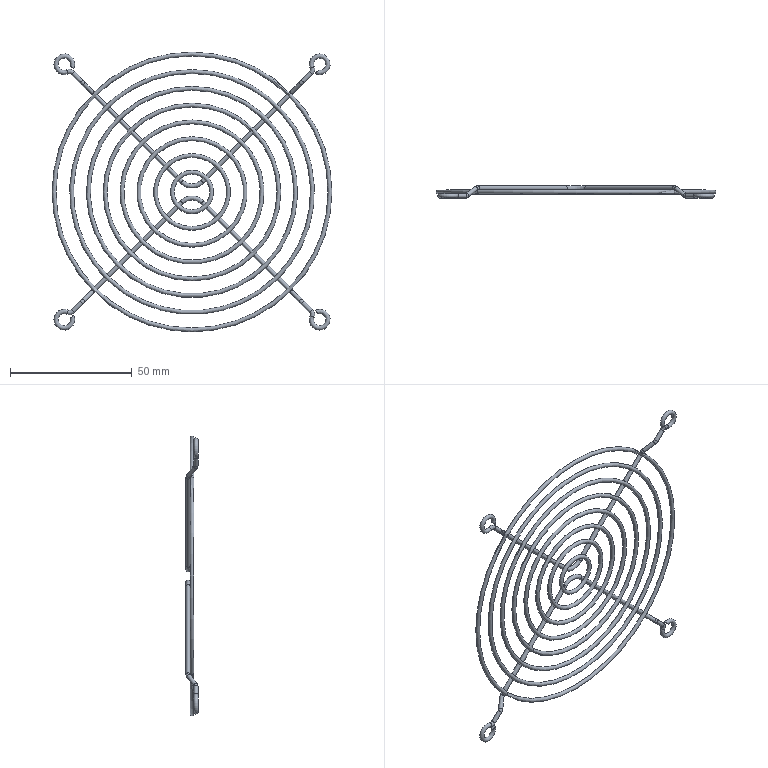Part | STEP file | E-SFG-120-R | 1 solid | 42 faces | box 115 x 5 x 115 mm | volume 4127 mm3 | torus 26 | cylinder 12 | plane 4 | commonest cylinder face diameters 1.75 x12